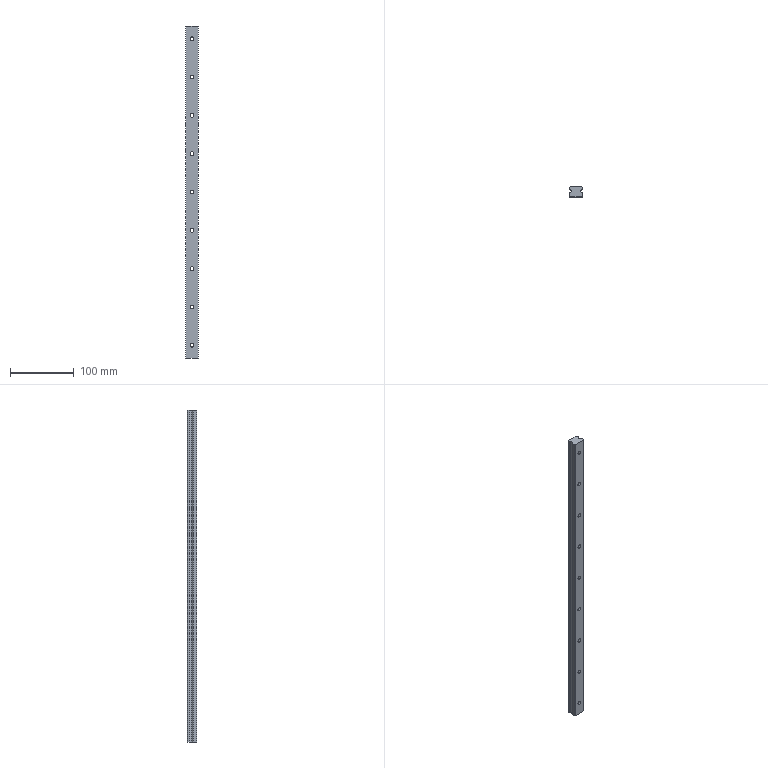Part | STEP file | 0243_Z_SXR28-520_1 | 1 solid | 62 faces | box 20 x 15.5 x 520 mm | volume 142241 mm3 | cylinder 41 | plane 21 | commonest cylinder face diameters 6 x18 9.5 x18 5 x3 3 x2